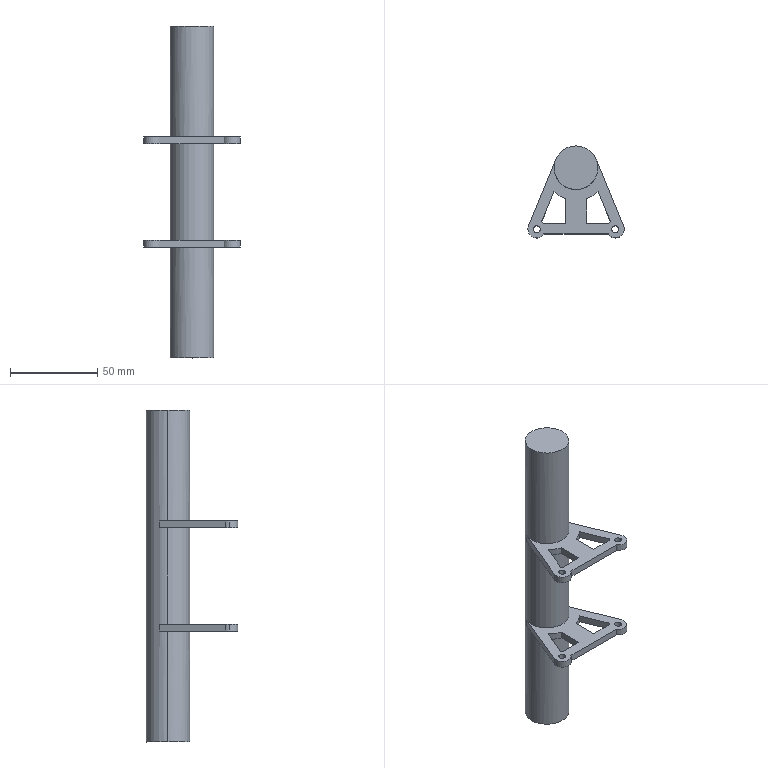Part | STEP file | Frame_Brackets | 1 solid | 50 faces | box 55 x 52.5 x 189.816 mm | volume 101287 mm3 | cylinder 26 | plane 24 | commonest cylinder face diameters 10 x10 4 x8 25 x4 37 x4